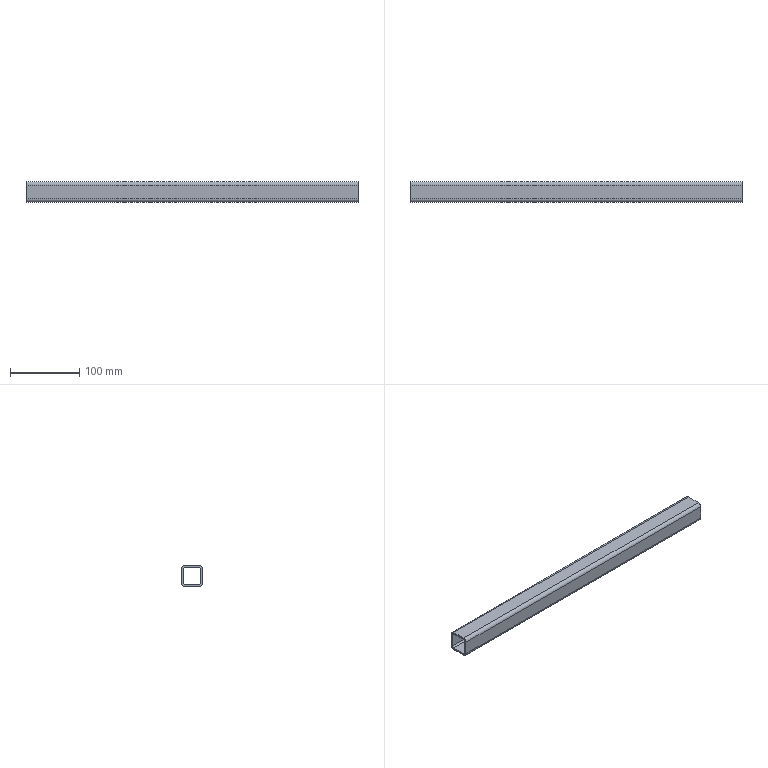Part | SolidWorks | features WeldMemberFeat 1, WeldmentFeature 1 | 1 solid | 18 faces | box 480 x 30 x 30 mm | volume 124274 mm3 | plane 10 | cylinder 8 | commonest cylinder face diameters 5 x4 10 x4
STEP:
#1=CARTESIAN_POINT('',(-240.,15.,10.));
#2=VERTEX_POINT('',#1);
#3=CARTESIAN_POINT('',(-240.,10.,15.));
#4=VERTEX_POINT('',#3);
#5=CARTESIAN_POINT('',(-240.,10.,10.));
#6=DIRECTION('',(1.,0.,0.));
#7=DIRECTION('',(0.,1.,0.));
#8=AXIS2_PLACEMENT_3D('',#5,#6,#7);
#9=CIRCLE('',#8,5.);
#10=EDGE_CURVE('',#2,#4,#9,.T.);
#11=ORIENTED_EDGE('',*,*,#10,.T.);
#12=CARTESIAN_POINT('',(240.,10.,15.));
#13=VERTEX_POINT('',#12);
#14=CARTESIAN_POINT('',(240.,10.,15.));
#15=DIRECTION('',(-1.,0.,0.));
#16=VECTOR('',#15,1000.);
#17=LINE('',#14,#16);
#18=EDGE_CURVE('',#13,#4,#17,.T.);
#19=ORIENTED_EDGE('',*,*,#18,.F.);
#20=CARTESIAN_POINT('',(240.,15.,10.));
#21=VERTEX_POINT('',#20);
#22=CARTESIAN_POINT('',(240.,10.,10.));
#23=DIRECTION('',(1.,0.,0.));
#24=DIRECTION('',(0.,1.,0.));
#25=AXIS2_PLACEMENT_3D('',#22,#23,#24);
#26=CIRCLE('',#25,5.);
#27=EDGE_CURVE('',#21,#13,#26,.T.);
#28=ORIENTED_EDGE('',*,*,#27,.F.);
#29=CARTESIAN_POINT('',(240.,15.,10.));
#30=DIRECTION('',(-1.,0.,0.));
#31=VECTOR('',#30,1000.);
#32=LINE('',#29,#31);
#33=EDGE_CURVE('',#21,#2,#32,.T.);
#34=ORIENTED_EDGE('',*,*,#33,.T.);
#35=EDGE_LOOP('',(#11,#19,#28,#34));
#36=FACE_OUTER_BOUND('',#35,.T.);
#37=CARTESIAN_POINT('',(240.,10.,10.));
#38=DIRECTION('',(-1.,0.,0.));
#39=DIRECTION('',(0.,-1.,0.));
#40=AXIS2_PLACEMENT_3D('',#37,#38,#39);
#41=CYLINDRICAL_SURFACE('',#40,5.);
#42=ADVANCED_FACE('',(#36),#41,.T.);
#43=CARTESIAN_POINT('',(-240.,-10.,15.));
#44=VERTEX_POINT('',#43);
#45=CARTESIAN_POINT('',(-240.,10.,15.));
#46=DIRECTION('',(0.,-1.,0.));
#47=VECTOR('',#46,1000.);
#48=LINE('',#45,#47);
#49=EDGE_CURVE('',#4,#44,#48,.T.);
#50=ORIENTED_EDGE('',*,*,#49,.T.);
#51=CARTESIAN_POINT('',(240.,-10.,15.));
#52=VERTEX_POINT('',#51);
#53=CARTESIAN_POINT('',(240.,-10.,15.));
#54=DIRECTION('',(-1.,0.,0.));
#55=VECTOR('',#54,1000.);
#56=LINE('',#53,#55);
#57=EDGE_CURVE('',#52,#44,#56,.T.);
#58=ORIENTED_EDGE('',*,*,#57,.F.);
#59=CARTESIAN_POINT('',(240.,10.,15.));
#60=DIRECTION('',(0.,-1.,0.));
#61=VECTOR('',#60,1000.);
#62=LINE('',#59,#61);
#63=EDGE_CURVE('',#13,#52,#62,.T.);
#64=ORIENTED_EDGE('',*,*,#63,.F.);
#65=ORIENTED_EDGE('',*,*,#18,.T.);
#66=EDGE_LOOP('',(#50,#58,#64,#65));
#67=FACE_OUTER_BOUND('',#66,.T.);
#68=CARTESIAN_POINT('',(240.,10.,15.));
#69=DIRECTION('',(0.,0.,-1.));
#70=DIRECTION('',(-1.,0.,0.));
#71=AXIS2_PLACEMENT_3D('',#68,#69,#70);
#72=PLANE('',#71);
#73=ADVANCED_FACE('',(#67),#72,.F.);
#74=CARTESIAN_POINT('',(-240.,-15.,10.));
#75=VERTEX_POINT('',#74);
#76=CARTESIAN_POINT('',(-240.,-10.,10.));
#77=DIRECTION('',(1.,0.,0.));
#78=DIRECTION('',(0.,1.,0.));
#79=AXIS2_PLACEMENT_3D('',#76,#77,#78);
#80=CIRCLE('',#79,5.);
#81=EDGE_CURVE('',#44,#75,#80,.T.);
#82=ORIENTED_EDGE('',*,*,#81,.T.);
#83=CARTESIAN_POINT('',(240.,-15.,10.));
#84=VERTEX_POINT('',#83);
#85=CARTESIAN_POINT('',(240.,-15.,10.));
#86=DIRECTION('',(-1.,0.,0.));
#87=VECTOR('',#86,1000.);
#88=LINE('',#85,#87);
#89=EDGE_CURVE('',#84,#75,#88,.T.);
#90=ORIENTED_EDGE('',*,*,#89,.F.);
#91=CARTESIAN_POINT('',(240.,-10.,10.));
#92=DIRECTION('',(1.,0.,0.));
#93=DIRECTION('',(0.,1.,0.));
#94=AXIS2_PLACEMENT_3D('',#91,#92,#93);
#95=CIRCLE('',#94,5.);
#96=EDGE_CURVE('',#52,#84,#95,.T.);
#97=ORIENTED_EDGE('',*,*,#96,.F.);
#98=ORIENTED_EDGE('',*,*,#57,.T.);
#99=EDGE_LOOP('',(#82,#90,#97,#98));
#100=FACE_OUTER_BOUND('',#99,.T.);
#101=CARTESIAN_POINT('',(240.,-10.,10.));
#102=DIRECTION('',(-1.,0.,0.));
#103=DIRECTION('',(0.,-1.,0.));
#104=AXIS2_PLACEMENT_3D('',#101,#102,#103);
#105=CYLINDRICAL_SURFACE('',#104,5.);
#106=ADVANCED_FACE('',(#100),#105,.T.);
#107=CARTESIAN_POINT('',(-240.,-15.,-10.));
#108=VERTEX_POINT('',#107);
#109=CARTESIAN_POINT('',(-240.,-15.,-10.));
#110=DIRECTION('',(0.,0.,-1.));
#111=VECTOR('',#110,1000.);
#112=LINE('',#109,#111);
#113=EDGE_CURVE('',#75,#108,#112,.T.);
#114=ORIENTED_EDGE('',*,*,#113,.T.);
#115=CARTESIAN_POINT('',(240.,-15.,-10.));
#116=VERTEX_POINT('',#115);
#117=CARTESIAN_POINT('',(240.,-15.,-10.));
#118=DIRECTION('',(-1.,0.,0.));
#119=VECTOR('',#118,1000.);
#120=LINE('',#117,#119);
#121=EDGE_CURVE('',#116,#108,#120,.T.);
#122=ORIENTED_EDGE('',*,*,#121,.F.);
#123=CARTESIAN_POINT('',(240.,-15.,-10.));
#124=DIRECTION('',(0.,0.,-1.));
#125=VECTOR('',#124,1000.);
#126=LINE('',#123,#125);
#127=EDGE_CURVE('',#84,#116,#126,.T.);
#128=ORIENTED_EDGE('',*,*,#127,.F.);
#129=ORIENTED_EDGE('',*,*,#89,.T.);
#130=EDGE_LOOP('',(#114,#122,#128,#129));
#131=FACE_OUTER_BOUND('',#130,.T.);
#132=CARTESIAN_POINT('',(240.,-15.,-10.));
#133=DIRECTION('',(0.,1.,0.));
#134=DIRECTION('',(-1.,0.,0.));
#135=AXIS2_PLACEMENT_3D('',#132,#133,#134);
#136=PLANE('',#135);
#137=ADVANCED_FACE('',(#131),#136,.F.);
#138=CARTESIAN_POINT('',(-240.,-10.,-15.));
#139=VERTEX_POINT('',#138);
#140=CARTESIAN_POINT('',(-240.,-10.,-10.));
#141=DIRECTION('',(1.,0.,0.));
#142=DIRECTION('',(0.,1.,0.));
#143=AXIS2_PLACEMENT_3D('',#140,#141,#142);
#144=CIRCLE('',#143,5.);
#145=EDGE_CURVE('',#108,#139,#144,.T.);
#146=ORIENTED_EDGE('',*,*,#145,.T.);
#147=CARTESIAN_POINT('',(240.,-10.,-15.));
#148=VERTEX_POINT('',#147);
#149=CARTESIAN_POINT('',(240.,-10.,-15.));
#150=DIRECTION('',(-1.,0.,0.));
#151=VECTOR('',#150,1000.);
#152=LINE('',#149,#151);
#153=EDGE_CURVE('',#148,#139,#152,.T.);
#154=ORIENTED_EDGE('',*,*,#153,.F.);
#155=CARTESIAN_POINT('',(240.,-10.,-10.));
#156=DIRECTION('',(1.,0.,0.));
#157=DIRECTION('',(0.,1.,0.));
#158=AXIS2_PLACEMENT_3D('',#155,#156,#157);
#159=CIRCLE('',#158,5.);
#160=EDGE_CURVE('',#116,#148,#159,.T.);
#161=ORIENTED_EDGE('',*,*,#160,.F.);
#162=ORIENTED_EDGE('',*,*,#121,.T.);
#163=EDGE_LOOP('',(#146,#154,#161,#162));
#164=FACE_OUTER_BOUND('',#163,.T.);
#165=CARTESIAN_POINT('',(240.,-10.,-10.));
#166=DIRECTION('',(-1.,0.,0.));
#167=DIRECTION('',(0.,-1.,0.));
#168=AXIS2_PLACEMENT_3D('',#165,#166,#167);
#169=CYLINDRICAL_SURFACE('',#168,5.);
#170=ADVANCED_FACE('',(#164),#169,.T.);
#171=CARTESIAN_POINT('',(-240.,10.,-15.));
#172=VERTEX_POINT('',#171);
#173=CARTESIAN_POINT('',(-240.,-10.,-15.));
#174=DIRECTION('',(0.,1.,0.));
#175=VECTOR('',#174,1000.);
#176=LINE('',#173,#175);
#177=EDGE_CURVE('',#139,#172,#176,.T.);
#178=ORIENTED_EDGE('',*,*,#177,.T.);
#179=CARTESIAN_POINT('',(240.,10.,-15.));
#180=VERTEX_POINT('',#179);
#181=CARTESIAN_POINT('',(240.,10.,-15.));
#182=DIRECTION('',(-1.,0.,0.));
#183=VECTOR('',#182,1000.);
#184=LINE('',#181,#183);
#185=EDGE_CURVE('',#180,#172,#184,.T.);
#186=ORIENTED_EDGE('',*,*,#185,.F.);
#187=CARTESIAN_POINT('',(240.,-10.,-15.));
#188=DIRECTION('',(0.,1.,0.));
#189=VECTOR('',#188,1000.);
#190=LINE('',#187,#189);
#191=EDGE_CURVE('',#148,#180,#190,.T.);
#192=ORIENTED_EDGE('',*,*,#191,.F.);
#193=ORIENTED_EDGE('',*,*,#153,.T.);
#194=EDGE_LOOP('',(#178,#186,#192,#193));
#195=FACE_OUTER_BOUND('',#194,.T.);
#196=CARTESIAN_POINT('',(240.,-10.,-15.));
#197=DIRECTION('',(0.,0.,1.));
#198=DIRECTION('',(1.,0.,0.));
#199=AXIS2_PLACEMENT_3D('',#196,#197,#198);
#200=PLANE('',#199);
#201=ADVANCED_FACE('',(#195),#200,.F.);
#202=CARTESIAN_POINT('',(-240.,15.,-10.));
#203=VERTEX_POINT('',#202);
#204=CARTESIAN_POINT('',(-240.,10.,-10.));
#205=DIRECTION('',(1.,0.,0.));
#206=DIRECTION('',(0.,1.,0.));
#207=AXIS2_PLACEMENT_3D('',#204,#205,#206);
#208=CIRCLE('',#207,5.);
#209=EDGE_CURVE('',#172,#203,#208,.T.);
#210=ORIENTED_EDGE('',*,*,#209,.T.);
#211=CARTESIAN_POINT('',(240.,15.,-10.));
#212=VERTEX_POINT('',#211);
#213=CARTESIAN_POINT('',(240.,15.,-10.));
#214=DIRECTION('',(-1.,0.,0.));
#215=VECTOR('',#214,1000.);
#216=LINE('',#213,#215);
#217=EDGE_CURVE('',#212,#203,#216,.T.);
#218=ORIENTED_EDGE('',*,*,#217,.F.);
#219=CARTESIAN_POINT('',(240.,10.,-10.));
#220=DIRECTION('',(1.,0.,0.));
#221=DIRECTION('',(0.,1.,0.));
#222=AXIS2_PLACEMENT_3D('',#219,#220,#221);
#223=CIRCLE('',#222,5.);
#224=EDGE_CURVE('',#180,#212,#223,.T.);
#225=ORIENTED_EDGE('',*,*,#224,.F.);
#226=ORIENTED_EDGE('',*,*,#185,.T.);
#227=EDGE_LOOP('',(#210,#218,#225,#226));
#228=FACE_OUTER_BOUND('',#227,.T.);
#229=CARTESIAN_POINT('',(240.,10.,-10.));
#230=DIRECTION('',(-1.,0.,0.));
#231=DIRECTION('',(0.,-1.,0.));
#232=AXIS2_PLACEMENT_3D('',#229,#230,#231);
#233=CYLINDRICAL_SURFACE('',#232,5.);
#234=ADVANCED_FACE('',(#228),#233,.T.);
#235=CARTESIAN_POINT('',(-240.,-10.,12.5));
#236=VERTEX_POINT('',#235);
#237=CARTESIAN_POINT('',(-240.,-12.5,10.));
#238=VERTEX_POINT('',#237);
#239=CARTESIAN_POINT('',(-240.,-10.,10.));
#240=DIRECTION('',(1.,0.,0.));
#241=DIRECTION('',(0.,1.,0.));
#242=AXIS2_PLACEMENT_3D('',#239,#240,#241);
#243=CIRCLE('',#242,2.5);
#244=EDGE_CURVE('',#236,#238,#243,.T.);
#245=ORIENTED_EDGE('',*,*,#244,.F.);
#246=CARTESIAN_POINT('',(240.,-10.,12.5));
#247=VERTEX_POINT('',#246);
#248=CARTESIAN_POINT('',(240.,-10.,12.5));
#249=DIRECTION('',(-1.,0.,0.));
#250=VECTOR('',#249,1000.);
#251=LINE('',#248,#250);
#252=EDGE_CURVE('',#247,#236,#251,.T.);
#253=ORIENTED_EDGE('',*,*,#252,.F.);
#254=CARTESIAN_POINT('',(240.,-12.5,10.));
#255=VERTEX_POINT('',#254);
#256=CARTESIAN_POINT('',(240.,-10.,10.));
#257=DIRECTION('',(1.,0.,0.));
#258=DIRECTION('',(0.,1.,0.));
#259=AXIS2_PLACEMENT_3D('',#256,#257,#258);
#260=CIRCLE('',#259,2.5);
#261=EDGE_CURVE('',#247,#255,#260,.T.);
#262=ORIENTED_EDGE('',*,*,#261,.T.);
#263=CARTESIAN_POINT('',(240.,-12.5,10.));
#264=DIRECTION('',(-1.,0.,0.));
#265=VECTOR('',#264,1000.);
#266=LINE('',#263,#265);
#267=EDGE_CURVE('',#255,#238,#266,.T.);
#268=ORIENTED_EDGE('',*,*,#267,.T.);
#269=EDGE_LOOP('',(#245,#253,#262,#268));
#270=FACE_OUTER_BOUND('',#269,.T.);
#271=CARTESIAN_POINT('',(240.,-10.,10.));
#272=DIRECTION('',(-1.,0.,0.));
#273=DIRECTION('',(0.,-1.,0.));
#274=AXIS2_PLACEMENT_3D('',#271,#272,#273);
#275=CYLINDRICAL_SURFACE('',#274,2.5);
#276=ADVANCED_FACE('',(#270),#275,.F.);
#277=CARTESIAN_POINT('',(-240.,10.,12.5));
#278=VERTEX_POINT('',#277);
#279=CARTESIAN_POINT('',(-240.,10.,12.5));
#280=DIRECTION('',(0.,-1.,0.));
#281=VECTOR('',#280,1000.);
#282=LINE('',#279,#281);
#283=EDGE_CURVE('',#278,#236,#282,.T.);
#284=ORIENTED_EDGE('',*,*,#283,.F.);
#285=CARTESIAN_POINT('',(240.,10.,12.5));
#286=VERTEX_POINT('',#285);
#287=CARTESIAN_POINT('',(240.,10.,12.5));
#288=DIRECTION('',(-1.,0.,0.));
#289=VECTOR('',#288,1000.);
#290=LINE('',#287,#289);
#291=EDGE_CURVE('',#286,#278,#290,.T.);
#292=ORIENTED_EDGE('',*,*,#291,.F.);
#293=CARTESIAN_POINT('',(240.,10.,12.5));
#294=DIRECTION('',(0.,-1.,0.));
#295=VECTOR('',#294,1000.);
#296=LINE('',#293,#295);
#297=EDGE_CURVE('',#286,#247,#296,.T.);
#298=ORIENTED_EDGE('',*,*,#297,.T.);
#299=ORIENTED_EDGE('',*,*,#252,.T.);
#300=EDGE_LOOP('',(#284,#292,#298,#299));
#301=FACE_OUTER_BOUND('',#300,.T.);
#302=CARTESIAN_POINT('',(240.,10.,12.5));
#303=DIRECTION('',(0.,0.,-1.));
#304=DIRECTION('',(-1.,0.,0.));
#305=AXIS2_PLACEMENT_3D('',#302,#303,#304);
#306=PLANE('',#305);
#307=ADVANCED_FACE('',(#301),#306,.T.);
#308=CARTESIAN_POINT('',(-240.,12.5,10.));
#309=VERTEX_POINT('',#308);
#310=CARTESIAN_POINT('',(-240.,10.,10.));
#311=DIRECTION('',(1.,0.,0.));
#312=DIRECTION('',(0.,1.,0.));
#313=AXIS2_PLACEMENT_3D('',#310,#311,#312);
#314=CIRCLE('',#313,2.5);
#315=EDGE_CURVE('',#309,#278,#314,.T.);
#316=ORIENTED_EDGE('',*,*,#315,.F.);
#317=CARTESIAN_POINT('',(240.,12.5,10.));
#318=VERTEX_POINT('',#317);
#319=CARTESIAN_POINT('',(240.,12.5,10.));
#320=DIRECTION('',(-1.,0.,0.));
#321=VECTOR('',#320,1000.);
#322=LINE('',#319,#321);
#323=EDGE_CURVE('',#318,#309,#322,.T.);
#324=ORIENTED_EDGE('',*,*,#323,.F.);
#325=CARTESIAN_POINT('',(240.,10.,10.));
#326=DIRECTION('',(1.,0.,0.));
#327=DIRECTION('',(0.,1.,0.));
#328=AXIS2_PLACEMENT_3D('',#325,#326,#327);
#329=CIRCLE('',#328,2.5);
#330=EDGE_CURVE('',#318,#286,#329,.T.);
#331=ORIENTED_EDGE('',*,*,#330,.T.);
#332=ORIENTED_EDGE('',*,*,#291,.T.);
#333=EDGE_LOOP('',(#316,#324,#331,#332));
#334=FACE_OUTER_BOUND('',#333,.T.);
#335=CARTESIAN_POINT('',(240.,10.,10.));
#336=DIRECTION('',(-1.,0.,0.));
#337=DIRECTION('',(0.,-1.,0.));
#338=AXIS2_PLACEMENT_3D('',#335,#336,#337);
#339=CYLINDRICAL_SURFACE('',#338,2.5);
#340=ADVANCED_FACE('',(#334),#339,.F.);
#341=CARTESIAN_POINT('',(-240.,12.5,-10.));
#342=VERTEX_POINT('',#341);
#343=CARTESIAN_POINT('',(-240.,12.5,10.));
#344=DIRECTION('',(0.,0.,1.));
#345=VECTOR('',#344,1000.);
#346=LINE('',#343,#345);
#347=EDGE_CURVE('',#342,#309,#346,.T.);
#348=ORIENTED_EDGE('',*,*,#347,.F.);
#349=CARTESIAN_POINT('',(240.,12.5,-10.));
#350=VERTEX_POINT('',#349);
#351=CARTESIAN_POINT('',(240.,12.5,-10.));
#352=DIRECTION('',(-1.,0.,0.));
#353=VECTOR('',#352,1000.);
#354=LINE('',#351,#353);
#355=EDGE_CURVE('',#350,#342,#354,.T.);
#356=ORIENTED_EDGE('',*,*,#355,.F.);
#357=CARTESIAN_POINT('',(240.,12.5,10.));
#358=DIRECTION('',(0.,0.,1.));
#359=VECTOR('',#358,1000.);
#360=LINE('',#357,#359);
#361=EDGE_CURVE('',#350,#318,#360,.T.);
#362=ORIENTED_EDGE('',*,*,#361,.T.);
#363=ORIENTED_EDGE('',*,*,#323,.T.);
#364=EDGE_LOOP('',(#348,#356,#362,#363));
#365=FACE_OUTER_BOUND('',#364,.T.);
#366=CARTESIAN_POINT('',(240.,12.5,10.));
#367=DIRECTION('',(0.,-1.,0.));
#368=DIRECTION('',(1.,0.,0.));
#369=AXIS2_PLACEMENT_3D('',#366,#367,#368);
#370=PLANE('',#369);
#371=ADVANCED_FACE('',(#365),#370,.T.);
#372=CARTESIAN_POINT('',(-240.,10.,-12.5));
#373=VERTEX_POINT('',#372);
#374=CARTESIAN_POINT('',(-240.,10.,-10.));
#375=DIRECTION('',(1.,0.,0.));
#376=DIRECTION('',(0.,1.,0.));
#377=AXIS2_PLACEMENT_3D('',#374,#375,#376);
#378=CIRCLE('',#377,2.5);
#379=EDGE_CURVE('',#373,#342,#378,.T.);
#380=ORIENTED_EDGE('',*,*,#379,.F.);
#381=CARTESIAN_POINT('',(240.,10.,-12.5));
#382=VERTEX_POINT('',#381);
#383=CARTESIAN_POINT('',(240.,10.,-12.5));
#384=DIRECTION('',(-1.,0.,0.));
#385=VECTOR('',#384,1000.);
#386=LINE('',#383,#385);
#387=EDGE_CURVE('',#382,#373,#386,.T.);
#388=ORIENTED_EDGE('',*,*,#387,.F.);
#389=CARTESIAN_POINT('',(240.,10.,-10.));
#390=DIRECTION('',(1.,0.,0.));
#391=DIRECTION('',(0.,1.,0.));
#392=AXIS2_PLACEMENT_3D('',#389,#390,#391);
#393=CIRCLE('',#392,2.5);
#394=EDGE_CURVE('',#382,#350,#393,.T.);
#395=ORIENTED_EDGE('',*,*,#394,.T.);
#396=ORIENTED_EDGE('',*,*,#355,.T.);
#397=EDGE_LOOP('',(#380,#388,#395,#396));
#398=FACE_OUTER_BOUND('',#397,.T.);
#399=CARTESIAN_POINT('',(240.,10.,-10.));
#400=DIRECTION('',(-1.,0.,0.));
#401=DIRECTION('',(0.,-1.,0.));
#402=AXIS2_PLACEMENT_3D('',#399,#400,#401);
#403=CYLINDRICAL_SURFACE('',#402,2.5);
#404=ADVANCED_FACE('',(#398),#403,.F.);
#405=CARTESIAN_POINT('',(-240.,-10.,-12.5));
#406=VERTEX_POINT('',#405);
#407=CARTESIAN_POINT('',(-240.,-10.,-12.5));
#408=DIRECTION('',(0.,1.,0.));
#409=VECTOR('',#408,1000.);
#410=LINE('',#407,#409);
#411=EDGE_CURVE('',#406,#373,#410,.T.);
#412=ORIENTED_EDGE('',*,*,#411,.F.);
#413=CARTESIAN_POINT('',(240.,-10.,-12.5));
#414=VERTEX_POINT('',#413);
#415=CARTESIAN_POINT('',(240.,-10.,-12.5));
#416=DIRECTION('',(-1.,0.,0.));
#417=VECTOR('',#416,1000.);
#418=LINE('',#415,#417);
#419=EDGE_CURVE('',#414,#406,#418,.T.);
#420=ORIENTED_EDGE('',*,*,#419,.F.);
#421=CARTESIAN_POINT('',(240.,-10.,-12.5));
#422=DIRECTION('',(0.,1.,0.));
#423=VECTOR('',#422,1000.);
#424=LINE('',#421,#423);
#425=EDGE_CURVE('',#414,#382,#424,.T.);
#426=ORIENTED_EDGE('',*,*,#425,.T.);
#427=ORIENTED_EDGE('',*,*,#387,.T.);
#428=EDGE_LOOP('',(#412,#420,#426,#427));
#429=FACE_OUTER_BOUND('',#428,.T.);
#430=CARTESIAN_POINT('',(240.,-10.,-12.5));
#431=DIRECTION('',(0.,0.,1.));
#432=DIRECTION('',(1.,0.,0.));
#433=AXIS2_PLACEMENT_3D('',#430,#431,#432);
#434=PLANE('',#433);
#435=ADVANCED_FACE('',(#429),#434,.T.);
#436=CARTESIAN_POINT('',(-240.,-12.5,-10.));
#437=VERTEX_POINT('',#436);
#438=CARTESIAN_POINT('',(-240.,-10.,-10.));
#439=DIRECTION('',(1.,0.,0.));
#440=DIRECTION('',(0.,1.,0.));
#441=AXIS2_PLACEMENT_3D('',#438,#439,#440);
#442=CIRCLE('',#441,2.5);
#443=EDGE_CURVE('',#437,#406,#442,.T.);
#444=ORIENTED_EDGE('',*,*,#443,.F.);
#445=CARTESIAN_POINT('',(240.,-12.5,-10.));
#446=VERTEX_POINT('',#445);
#447=CARTESIAN_POINT('',(240.,-12.5,-10.));
#448=DIRECTION('',(-1.,0.,0.));
#449=VECTOR('',#448,1000.);
#450=LINE('',#447,#449);
#451=EDGE_CURVE('',#446,#437,#450,.T.);
#452=ORIENTED_EDGE('',*,*,#451,.F.);
#453=CARTESIAN_POINT('',(240.,-10.,-10.));
#454=DIRECTION('',(1.,0.,0.));
#455=DIRECTION('',(0.,1.,0.));
#456=AXIS2_PLACEMENT_3D('',#453,#454,#455);
#457=CIRCLE('',#456,2.5);
#458=EDGE_CURVE('',#446,#414,#457,.T.);
#459=ORIENTED_EDGE('',*,*,#458,.T.);
#460=ORIENTED_EDGE('',*,*,#419,.T.);
#461=EDGE_LOOP('',(#444,#452,#459,#460));
#462=FACE_OUTER_BOUND('',#461,.T.);
#463=CARTESIAN_POINT('',(240.,-10.,-10.));
#464=DIRECTION('',(-1.,0.,0.));
#465=DIRECTION('',(0.,-1.,0.));
#466=AXIS2_PLACEMENT_3D('',#463,#464,#465);
#467=CYLINDRICAL_SURFACE('',#466,2.5);
#468=ADVANCED_FACE('',(#462),#467,.F.);
#469=CARTESIAN_POINT('',(-240.,-12.5,-10.));
#470=DIRECTION('',(0.,0.,-1.));
#471=VECTOR('',#470,1000.);
#472=LINE('',#469,#471);
#473=EDGE_CURVE('',#238,#437,#472,.T.);
#474=ORIENTED_EDGE('',*,*,#473,.F.);
#475=ORIENTED_EDGE('',*,*,#267,.F.);
#476=CARTESIAN_POINT('',(240.,-12.5,-10.));
#477=DIRECTION('',(0.,0.,-1.));
#478=VECTOR('',#477,1000.);
#479=LINE('',#476,#478);
#480=EDGE_CURVE('',#255,#446,#479,.T.);
#481=ORIENTED_EDGE('',*,*,#480,.T.);
#482=ORIENTED_EDGE('',*,*,#451,.T.);
#483=EDGE_LOOP('',(#474,#475,#481,#482));
#484=FACE_OUTER_BOUND('',#483,.T.);
#485=CARTESIAN_POINT('',(240.,-12.5,-10.));
#486=DIRECTION('',(0.,1.,0.));
#487=DIRECTION('',(-1.,0.,0.));
#488=AXIS2_PLACEMENT_3D('',#485,#486,#487);
#489=PLANE('',#488);
#490=ADVANCED_FACE('',(#484),#489,.T.);
#491=CARTESIAN_POINT('',(-240.,15.,10.));
#492=DIRECTION('',(0.,0.,1.));
#493=VECTOR('',#492,1000.);
#494=LINE('',#491,#493);
#495=EDGE_CURVE('',#203,#2,#494,.T.);
#496=ORIENTED_EDGE('',*,*,#495,.T.);
#497=ORIENTED_EDGE('',*,*,#33,.F.);
#498=CARTESIAN_POINT('',(240.,15.,10.));
#499=DIRECTION('',(0.,0.,1.));
#500=VECTOR('',#499,1000.);
#501=LINE('',#498,#500);
#502=EDGE_CURVE('',#212,#21,#501,.T.);
#503=ORIENTED_EDGE('',*,*,#502,.F.);
#504=ORIENTED_EDGE('',*,*,#217,.T.);
#505=EDGE_LOOP('',(#496,#497,#503,#504));
#506=FACE_OUTER_BOUND('',#505,.T.);
#507=CARTESIAN_POINT('',(240.,15.,10.));
#508=DIRECTION('',(0.,-1.,0.));
#509=DIRECTION('',(1.,0.,0.));
#510=AXIS2_PLACEMENT_3D('',#507,#508,#509);
#511=PLANE('',#510);
#512=ADVANCED_FACE('',(#506),#511,.F.);
#513=ORIENTED_EDGE('',*,*,#261,.F.);
#514=ORIENTED_EDGE('',*,*,#297,.F.);
#515=ORIENTED_EDGE('',*,*,#330,.F.);
#516=ORIENTED_EDGE('',*,*,#361,.F.);
#517=ORIENTED_EDGE('',*,*,#394,.F.);
#518=ORIENTED_EDGE('',*,*,#425,.F.);
#519=ORIENTED_EDGE('',*,*,#458,.F.);
#520=ORIENTED_EDGE('',*,*,#480,.F.);
#521=EDGE_LOOP('',(#513,#514,#515,#516,#517,#518,#519,#520));
#522=FACE_BOUND('',#521,.T.);
#523=ORIENTED_EDGE('',*,*,#27,.T.);
#524=ORIENTED_EDGE('',*,*,#63,.T.);
#525=ORIENTED_EDGE('',*,*,#96,.T.);
#526=ORIENTED_EDGE('',*,*,#127,.T.);
#527=ORIENTED_EDGE('',*,*,#160,.T.);
#528=ORIENTED_EDGE('',*,*,#191,.T.);
#529=ORIENTED_EDGE('',*,*,#224,.T.);
#530=ORIENTED_EDGE('',*,*,#502,.T.);
#531=EDGE_LOOP('',(#523,#524,#525,#526,#527,#528,#529,#530));
#532=FACE_OUTER_BOUND('',#531,.T.);
#533=CARTESIAN_POINT('',(240.,10.,10.));
#534=DIRECTION('',(1.,0.,0.));
#535=DIRECTION('',(0.,1.,0.));
#536=AXIS2_PLACEMENT_3D('',#533,#534,#535);
#537=PLANE('',#536);
#538=ADVANCED_FACE('',(#522,#532),#537,.T.);
#539=ORIENTED_EDGE('',*,*,#244,.T.);
#540=ORIENTED_EDGE('',*,*,#473,.T.);
#541=ORIENTED_EDGE('',*,*,#443,.T.);
#542=ORIENTED_EDGE('',*,*,#411,.T.);
#543=ORIENTED_EDGE('',*,*,#379,.T.);
#544=ORIENTED_EDGE('',*,*,#347,.T.);
#545=ORIENTED_EDGE('',*,*,#315,.T.);
#546=ORIENTED_EDGE('',*,*,#283,.T.);
#547=EDGE_LOOP('',(#539,#540,#541,#542,#543,#544,#545,#546));
#548=FACE_BOUND('',#547,.T.);
#549=ORIENTED_EDGE('',*,*,#10,.F.);
#550=ORIENTED_EDGE('',*,*,#495,.F.);
#551=ORIENTED_EDGE('',*,*,#209,.F.);
#552=ORIENTED_EDGE('',*,*,#177,.F.);
#553=ORIENTED_EDGE('',*,*,#145,.F.);
#554=ORIENTED_EDGE('',*,*,#113,.F.);
#555=ORIENTED_EDGE('',*,*,#81,.F.);
#556=ORIENTED_EDGE('',*,*,#49,.F.);
#557=EDGE_LOOP('',(#549,#550,#551,#552,#553,#554,#555,#556));
#558=FACE_OUTER_BOUND('',#557,.T.);
#559=CARTESIAN_POINT('',(-240.,10.,10.));
#560=DIRECTION('',(1.,0.,0.));
#561=DIRECTION('',(0.,1.,0.));
#562=AXIS2_PLACEMENT_3D('',#559,#560,#561);
#563=PLANE('',#562);
#564=ADVANCED_FACE('',(#548,#558),#563,.F.);
#565=CLOSED_SHELL('',(#42,#73,#106,#137,#170,#201,#234,#276,#307,#340,#371,#404,#435,#468,#490,#512,#538,#564));
#566=MANIFOLD_SOLID_BREP('',#565);
#567=CARTESIAN_POINT('',(0.,0.,0.));
#568=DIRECTION('',(0.,0.,1.));
#569=DIRECTION('',(1.,0.,0.));
#570=AXIS2_PLACEMENT_3D('',#567,#568,#569);
#571=(LENGTH_UNIT()NAMED_UNIT(*)SI_UNIT(.MILLI.,.METRE.));
#572=UNCERTAINTY_MEASURE_WITH_UNIT(LENGTH_MEASURE(0.00001),#571,'','');
#573=(NAMED_UNIT(*)PLANE_ANGLE_UNIT()SI_UNIT($,.RADIAN.));
#574=(NAMED_UNIT(*)SI_UNIT($,.STERADIAN.)SOLID_ANGLE_UNIT());
#575=(GEOMETRIC_REPRESENTATION_CONTEXT(3)GLOBAL_UNCERTAINTY_ASSIGNED_CONTEXT((#572))GLOBAL_UNIT_ASSIGNED_CONTEXT((#571,#573,#574))REPRESENTATION_CONTEXT('',''));
#576=ADVANCED_BREP_SHAPE_REPRESENTATION('',(#566,#570),#575);